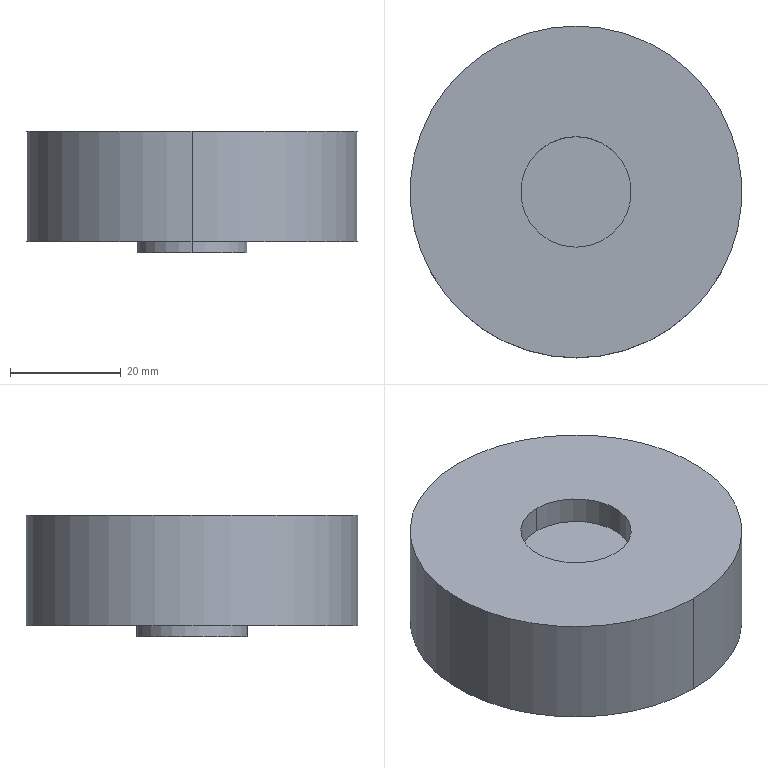Part | STEP file | B-PRF60 internal ring gear_first-stage internal ring gear | 1 solid | 10 faces | box 60 x 60 x 22 mm | volume 55606 mm3 | cylinder 6 | plane 4 | commonest cylinder face diameters 20 x4 60 x2
STEP:
#1=CARTESIAN_POINT('',(0.,0.,0.));
#2=DIRECTION('',(0.,0.,1.));
#3=DIRECTION('',(1.,0.,0.));
#4=AXIS2_PLACEMENT_3D('',#1,#2,#3);
#5=CARTESIAN_POINT('',(0.,-10.,-12.));
#6=VERTEX_POINT('',#5);
#7=CARTESIAN_POINT('',(0.,10.,-12.));
#8=VERTEX_POINT('',#7);
#9=CARTESIAN_POINT('',(0.,0.,-12.));
#10=DIRECTION('',(0.,0.,1.));
#11=DIRECTION('',(0.,-1.,0.));
#12=AXIS2_PLACEMENT_3D('',#9,#10,#11);
#13=CIRCLE('',#12,10.);
#14=CARTESIAN_POINT('',(0.,0.,-12.));
#15=DIRECTION('',(0.,0.,1.));
#16=DIRECTION('',(0.,-1.,0.));
#17=AXIS2_PLACEMENT_3D('',#14,#15,#16);
#18=CYLINDRICAL_SURFACE('',#17,10.);
#19=CARTESIAN_POINT('',(0.,0.));
#20=DIRECTION('',(1.,0.));
#21=VECTOR('',#20,1.);
#22=LINE('',#19,#21);
#23=(GEOMETRIC_REPRESENTATION_CONTEXT(2)PARAMETRIC_REPRESENTATION_CONTEXT()REPRESENTATION_CONTEXT('',''));
#24=DEFINITIONAL_REPRESENTATION('',(#22),#23);
#25=PCURVE('',#18,#24);
#26=CARTESIAN_POINT('',(0.,0.,-12.));
#27=DIRECTION('',(0.,0.,-1.));
#28=DIRECTION('',(-1.,0.,0.));
#29=AXIS2_PLACEMENT_3D('',#26,#27,#28);
#30=PLANE('',#29);
#31=CARTESIAN_POINT('',(0.,-10.));
#32=CARTESIAN_POINT('',(-17.321,-10.));
#33=CARTESIAN_POINT('',(-8.66,5.));
#34=CARTESIAN_POINT('',(0.,20.));
#35=CARTESIAN_POINT('',(8.66,5.));
#36=CARTESIAN_POINT('',(17.321,-10.));
#37=CARTESIAN_POINT('',(0.,-10.));
#38=(BOUNDED_CURVE()B_SPLINE_CURVE(2,(#31,#32,#33,#34,#35,#36,#37),.UNSPECIFIED.,.T.,.F.)B_SPLINE_CURVE_WITH_KNOTS((1,2,2,2,2,1),(-2.094,0.,2.094,4.189,6.283,8.378),.UNSPECIFIED.)CURVE()GEOMETRIC_REPRESENTATION_ITEM()RATIONAL_B_SPLINE_CURVE((1.,0.5,1.,0.5,1.,0.5,1.))REPRESENTATION_ITEM(''));
#39=(GEOMETRIC_REPRESENTATION_CONTEXT(2)PARAMETRIC_REPRESENTATION_CONTEXT()REPRESENTATION_CONTEXT('',''));
#40=DEFINITIONAL_REPRESENTATION('',(#38),#39);
#41=PCURVE('',#30,#40);
#42=SURFACE_CURVE('',#13,(#25,#41),.PCURVE_S1.);
#43=EDGE_CURVE('',#6,#8,#42,.T.);
#44=ORIENTED_EDGE('',*,*,#43,.T.);
#45=CARTESIAN_POINT('',(0.,10.,-10.));
#46=VERTEX_POINT('',#45);
#47=CARTESIAN_POINT('',(0.,10.,-12.));
#48=DIRECTION('',(0.,0.,1.));
#49=VECTOR('',#48,1.);
#50=LINE('',#47,#49);
#51=CARTESIAN_POINT('',(3.142,0.));
#52=DIRECTION('',(0.,1.));
#53=VECTOR('',#52,1.);
#54=LINE('',#51,#53);
#55=(GEOMETRIC_REPRESENTATION_CONTEXT(2)PARAMETRIC_REPRESENTATION_CONTEXT()REPRESENTATION_CONTEXT('',''));
#56=DEFINITIONAL_REPRESENTATION('',(#54),#55);
#57=PCURVE('',#18,#56);
#58=CARTESIAN_POINT('',(0.,0.,-12.));
#59=DIRECTION('',(0.,0.,1.));
#60=DIRECTION('',(0.,-1.,0.));
#61=AXIS2_PLACEMENT_3D('',#58,#59,#60);
#62=CYLINDRICAL_SURFACE('',#61,10.);
#63=CARTESIAN_POINT('',(3.142,0.));
#64=DIRECTION('',(0.,1.));
#65=VECTOR('',#64,1.);
#66=LINE('',#63,#65);
#67=(GEOMETRIC_REPRESENTATION_CONTEXT(2)PARAMETRIC_REPRESENTATION_CONTEXT()REPRESENTATION_CONTEXT('',''));
#68=DEFINITIONAL_REPRESENTATION('',(#66),#67);
#69=PCURVE('',#62,#68);
#70=SURFACE_CURVE('',#50,(#57,#69),.PCURVE_S1.);
#71=EDGE_CURVE('',#8,#46,#70,.T.);
#72=ORIENTED_EDGE('',*,*,#71,.T.);
#73=CARTESIAN_POINT('',(0.,-10.,-10.));
#74=VERTEX_POINT('',#73);
#75=CARTESIAN_POINT('',(0.,0.,-10.));
#76=DIRECTION('',(0.,0.,-1.));
#77=DIRECTION('',(0.,-1.,0.));
#78=AXIS2_PLACEMENT_3D('',#75,#76,#77);
#79=CIRCLE('',#78,10.);
#80=CARTESIAN_POINT('',(6.283,2.));
#81=DIRECTION('',(-1.,0.));
#82=VECTOR('',#81,1.);
#83=LINE('',#80,#82);
#84=(GEOMETRIC_REPRESENTATION_CONTEXT(2)PARAMETRIC_REPRESENTATION_CONTEXT()REPRESENTATION_CONTEXT('',''));
#85=DEFINITIONAL_REPRESENTATION('',(#83),#84);
#86=PCURVE('',#18,#85);
#87=CARTESIAN_POINT('',(0.,0.,-10.));
#88=DIRECTION('',(0.,0.,1.));
#89=DIRECTION('',(1.,0.,0.));
#90=AXIS2_PLACEMENT_3D('',#87,#88,#89);
#91=PLANE('',#90);
#92=CARTESIAN_POINT('',(0.,-10.));
#93=CARTESIAN_POINT('',(-17.321,-10.));
#94=CARTESIAN_POINT('',(-8.66,5.));
#95=CARTESIAN_POINT('',(0.,20.));
#96=CARTESIAN_POINT('',(8.66,5.));
#97=CARTESIAN_POINT('',(17.321,-10.));
#98=CARTESIAN_POINT('',(0.,-10.));
#99=(BOUNDED_CURVE()B_SPLINE_CURVE(2,(#92,#93,#94,#95,#96,#97,#98),.UNSPECIFIED.,.T.,.F.)B_SPLINE_CURVE_WITH_KNOTS((1,2,2,2,2,1),(-2.094,0.,2.094,4.189,6.283,8.378),.UNSPECIFIED.)CURVE()GEOMETRIC_REPRESENTATION_ITEM()RATIONAL_B_SPLINE_CURVE((1.,0.5,1.,0.5,1.,0.5,1.))REPRESENTATION_ITEM(''));
#100=(GEOMETRIC_REPRESENTATION_CONTEXT(2)PARAMETRIC_REPRESENTATION_CONTEXT()REPRESENTATION_CONTEXT('',''));
#101=DEFINITIONAL_REPRESENTATION('',(#99),#100);
#102=PCURVE('',#91,#101);
#103=SURFACE_CURVE('',#79,(#86,#102),.PCURVE_S1.);
#104=EDGE_CURVE('',#46,#74,#103,.T.);
#105=ORIENTED_EDGE('',*,*,#104,.T.);
#106=CARTESIAN_POINT('',(0.,-10.,-12.));
#107=DIRECTION('',(0.,0.,1.));
#108=VECTOR('',#107,1.);
#109=LINE('',#106,#108);
#110=CARTESIAN_POINT('',(0.,0.));
#111=DIRECTION('',(0.,1.));
#112=VECTOR('',#111,1.);
#113=LINE('',#110,#112);
#114=(GEOMETRIC_REPRESENTATION_CONTEXT(2)PARAMETRIC_REPRESENTATION_CONTEXT()REPRESENTATION_CONTEXT('',''));
#115=DEFINITIONAL_REPRESENTATION('',(#113),#114);
#116=PCURVE('',#18,#115);
#117=CARTESIAN_POINT('',(6.283,0.));
#118=DIRECTION('',(0.,1.));
#119=VECTOR('',#118,1.);
#120=LINE('',#117,#119);
#121=(GEOMETRIC_REPRESENTATION_CONTEXT(2)PARAMETRIC_REPRESENTATION_CONTEXT()REPRESENTATION_CONTEXT('',''));
#122=DEFINITIONAL_REPRESENTATION('',(#120),#121);
#123=PCURVE('',#62,#122);
#124=SURFACE_CURVE('',#109,(#116,#123),.PCURVE_S1.);
#125=EDGE_CURVE('',#6,#74,#124,.T.);
#126=ORIENTED_EDGE('',*,*,#125,.F.);
#127=EDGE_LOOP('',(#44,#72,#105,#126));
#128=FACE_BOUND('',#127,.T.);
#129=ADVANCED_FACE('',(#128),#18,.T.);
#130=CARTESIAN_POINT('',(0.,30.,10.));
#131=VERTEX_POINT('',#130);
#132=CARTESIAN_POINT('',(0.,-30.,10.));
#133=VERTEX_POINT('',#132);
#134=CARTESIAN_POINT('',(0.,0.,10.));
#135=DIRECTION('',(0.,0.,-1.));
#136=DIRECTION('',(0.,1.,0.));
#137=AXIS2_PLACEMENT_3D('',#134,#135,#136);
#138=CIRCLE('',#137,30.);
#139=CARTESIAN_POINT('',(0.,0.,10.));
#140=DIRECTION('',(0.,0.,-1.));
#141=DIRECTION('',(0.,1.,0.));
#142=AXIS2_PLACEMENT_3D('',#139,#140,#141);
#143=CYLINDRICAL_SURFACE('',#142,30.);
#144=CARTESIAN_POINT('',(0.,0.));
#145=DIRECTION('',(1.,0.));
#146=VECTOR('',#145,1.);
#147=LINE('',#144,#146);
#148=(GEOMETRIC_REPRESENTATION_CONTEXT(2)PARAMETRIC_REPRESENTATION_CONTEXT()REPRESENTATION_CONTEXT('',''));
#149=DEFINITIONAL_REPRESENTATION('',(#147),#148);
#150=PCURVE('',#143,#149);
#151=CARTESIAN_POINT('',(0.,0.,10.));
#152=DIRECTION('',(0.,0.,1.));
#153=DIRECTION('',(1.,0.,0.));
#154=AXIS2_PLACEMENT_3D('',#151,#152,#153);
#155=PLANE('',#154);
#156=CARTESIAN_POINT('',(0.,30.));
#157=CARTESIAN_POINT('',(51.962,30.));
#158=CARTESIAN_POINT('',(25.981,-15.));
#159=CARTESIAN_POINT('',(0.,-60.));
#160=CARTESIAN_POINT('',(-25.981,-15.));
#161=CARTESIAN_POINT('',(-51.962,30.));
#162=CARTESIAN_POINT('',(0.,30.));
#163=(BOUNDED_CURVE()B_SPLINE_CURVE(2,(#156,#157,#158,#159,#160,#161,#162),.UNSPECIFIED.,.T.,.F.)B_SPLINE_CURVE_WITH_KNOTS((1,2,2,2,2,1),(-2.094,0.,2.094,4.189,6.283,8.378),.UNSPECIFIED.)CURVE()GEOMETRIC_REPRESENTATION_ITEM()RATIONAL_B_SPLINE_CURVE((1.,0.5,1.,0.5,1.,0.5,1.))REPRESENTATION_ITEM(''));
#164=(GEOMETRIC_REPRESENTATION_CONTEXT(2)PARAMETRIC_REPRESENTATION_CONTEXT()REPRESENTATION_CONTEXT('',''));
#165=DEFINITIONAL_REPRESENTATION('',(#163),#164);
#166=PCURVE('',#155,#165);
#167=SURFACE_CURVE('',#138,(#150,#166),.PCURVE_S1.);
#168=EDGE_CURVE('',#131,#133,#167,.T.);
#169=ORIENTED_EDGE('',*,*,#168,.T.);
#170=CARTESIAN_POINT('',(0.,-30.,-10.));
#171=VERTEX_POINT('',#170);
#172=CARTESIAN_POINT('',(0.,-30.,10.));
#173=DIRECTION('',(0.,0.,-1.));
#174=VECTOR('',#173,1.);
#175=LINE('',#172,#174);
#176=CARTESIAN_POINT('',(3.142,0.));
#177=DIRECTION('',(0.,1.));
#178=VECTOR('',#177,1.);
#179=LINE('',#176,#178);
#180=(GEOMETRIC_REPRESENTATION_CONTEXT(2)PARAMETRIC_REPRESENTATION_CONTEXT()REPRESENTATION_CONTEXT('',''));
#181=DEFINITIONAL_REPRESENTATION('',(#179),#180);
#182=PCURVE('',#143,#181);
#183=CARTESIAN_POINT('',(0.,0.,10.));
#184=DIRECTION('',(0.,0.,-1.));
#185=DIRECTION('',(0.,1.,0.));
#186=AXIS2_PLACEMENT_3D('',#183,#184,#185);
#187=CYLINDRICAL_SURFACE('',#186,30.);
#188=CARTESIAN_POINT('',(3.142,0.));
#189=DIRECTION('',(0.,1.));
#190=VECTOR('',#189,1.);
#191=LINE('',#188,#190);
#192=(GEOMETRIC_REPRESENTATION_CONTEXT(2)PARAMETRIC_REPRESENTATION_CONTEXT()REPRESENTATION_CONTEXT('',''));
#193=DEFINITIONAL_REPRESENTATION('',(#191),#192);
#194=PCURVE('',#187,#193);
#195=SURFACE_CURVE('',#175,(#182,#194),.PCURVE_S1.);
#196=EDGE_CURVE('',#133,#171,#195,.T.);
#197=ORIENTED_EDGE('',*,*,#196,.T.);
#198=CARTESIAN_POINT('',(0.,30.,-10.));
#199=VERTEX_POINT('',#198);
#200=CARTESIAN_POINT('',(0.,0.,-10.));
#201=DIRECTION('',(0.,0.,1.));
#202=DIRECTION('',(0.,1.,0.));
#203=AXIS2_PLACEMENT_3D('',#200,#201,#202);
#204=CIRCLE('',#203,30.);
#205=CARTESIAN_POINT('',(6.283,20.));
#206=DIRECTION('',(-1.,0.));
#207=VECTOR('',#206,1.);
#208=LINE('',#205,#207);
#209=(GEOMETRIC_REPRESENTATION_CONTEXT(2)PARAMETRIC_REPRESENTATION_CONTEXT()REPRESENTATION_CONTEXT('',''));
#210=DEFINITIONAL_REPRESENTATION('',(#208),#209);
#211=PCURVE('',#143,#210);
#212=CARTESIAN_POINT('',(0.,0.));
#213=DIRECTION('',(0.,1.));
#214=AXIS2_PLACEMENT_2D('',#212,#213);
#215=CIRCLE('',#214,30.);
#216=(GEOMETRIC_REPRESENTATION_CONTEXT(2)PARAMETRIC_REPRESENTATION_CONTEXT()REPRESENTATION_CONTEXT('',''));
#217=DEFINITIONAL_REPRESENTATION('',(#215),#216);
#218=PCURVE('',#91,#217);
#219=SURFACE_CURVE('',#204,(#211,#218),.PCURVE_S1.);
#220=EDGE_CURVE('',#171,#199,#219,.T.);
#221=ORIENTED_EDGE('',*,*,#220,.T.);
#222=CARTESIAN_POINT('',(0.,30.,10.));
#223=DIRECTION('',(0.,0.,-1.));
#224=VECTOR('',#223,1.);
#225=LINE('',#222,#224);
#226=CARTESIAN_POINT('',(0.,0.));
#227=DIRECTION('',(0.,1.));
#228=VECTOR('',#227,1.);
#229=LINE('',#226,#228);
#230=(GEOMETRIC_REPRESENTATION_CONTEXT(2)PARAMETRIC_REPRESENTATION_CONTEXT()REPRESENTATION_CONTEXT('',''));
#231=DEFINITIONAL_REPRESENTATION('',(#229),#230);
#232=PCURVE('',#143,#231);
#233=CARTESIAN_POINT('',(6.283,0.));
#234=DIRECTION('',(0.,1.));
#235=VECTOR('',#234,1.);
#236=LINE('',#233,#235);
#237=(GEOMETRIC_REPRESENTATION_CONTEXT(2)PARAMETRIC_REPRESENTATION_CONTEXT()REPRESENTATION_CONTEXT('',''));
#238=DEFINITIONAL_REPRESENTATION('',(#236),#237);
#239=PCURVE('',#187,#238);
#240=SURFACE_CURVE('',#225,(#232,#239),.PCURVE_S1.);
#241=EDGE_CURVE('',#131,#199,#240,.T.);
#242=ORIENTED_EDGE('',*,*,#241,.F.);
#243=EDGE_LOOP('',(#169,#197,#221,#242));
#244=FACE_BOUND('',#243,.T.);
#245=ADVANCED_FACE('',(#244),#143,.T.);
#246=CARTESIAN_POINT('',(0.,-10.,5.));
#247=VERTEX_POINT('',#246);
#248=CARTESIAN_POINT('',(0.,-10.,10.));
#249=VERTEX_POINT('',#248);
#250=CARTESIAN_POINT('',(0.,-10.,5.));
#251=DIRECTION('',(0.,0.,1.));
#252=VECTOR('',#251,1.);
#253=LINE('',#250,#252);
#254=CARTESIAN_POINT('',(0.,0.,5.));
#255=DIRECTION('',(0.,0.,1.));
#256=DIRECTION('',(0.,-1.,0.));
#257=AXIS2_PLACEMENT_3D('',#254,#255,#256);
#258=CYLINDRICAL_SURFACE('',#257,10.);
#259=CARTESIAN_POINT('',(6.283,0.));
#260=DIRECTION('',(0.,1.));
#261=VECTOR('',#260,1.);
#262=LINE('',#259,#261);
#263=(GEOMETRIC_REPRESENTATION_CONTEXT(2)PARAMETRIC_REPRESENTATION_CONTEXT()REPRESENTATION_CONTEXT('',''));
#264=DEFINITIONAL_REPRESENTATION('',(#262),#263);
#265=PCURVE('',#258,#264);
#266=CARTESIAN_POINT('',(0.,0.,5.));
#267=DIRECTION('',(0.,0.,1.));
#268=DIRECTION('',(0.,-1.,0.));
#269=AXIS2_PLACEMENT_3D('',#266,#267,#268);
#270=CYLINDRICAL_SURFACE('',#269,10.);
#271=CARTESIAN_POINT('',(0.,0.));
#272=DIRECTION('',(0.,1.));
#273=VECTOR('',#272,1.);
#274=LINE('',#271,#273);
#275=(GEOMETRIC_REPRESENTATION_CONTEXT(2)PARAMETRIC_REPRESENTATION_CONTEXT()REPRESENTATION_CONTEXT('',''));
#276=DEFINITIONAL_REPRESENTATION('',(#274),#275);
#277=PCURVE('',#270,#276);
#278=SURFACE_CURVE('',#253,(#265,#277),.PCURVE_S1.);
#279=EDGE_CURVE('',#247,#249,#278,.T.);
#280=ORIENTED_EDGE('',*,*,#279,.T.);
#281=CARTESIAN_POINT('',(0.,10.,10.));
#282=VERTEX_POINT('',#281);
#283=CARTESIAN_POINT('',(0.,0.,10.));
#284=DIRECTION('',(0.,0.,-1.));
#285=DIRECTION('',(0.,-1.,0.));
#286=AXIS2_PLACEMENT_3D('',#283,#284,#285);
#287=CIRCLE('',#286,10.);
#288=CARTESIAN_POINT('',(6.283,5.));
#289=DIRECTION('',(-1.,0.));
#290=VECTOR('',#289,1.);
#291=LINE('',#288,#290);
#292=(GEOMETRIC_REPRESENTATION_CONTEXT(2)PARAMETRIC_REPRESENTATION_CONTEXT()REPRESENTATION_CONTEXT('',''));
#293=DEFINITIONAL_REPRESENTATION('',(#291),#292);
#294=PCURVE('',#258,#293);
#295=CARTESIAN_POINT('',(0.,-10.));
#296=CARTESIAN_POINT('',(-17.321,-10.));
#297=CARTESIAN_POINT('',(-8.66,5.));
#298=CARTESIAN_POINT('',(0.,20.));
#299=CARTESIAN_POINT('',(8.66,5.));
#300=CARTESIAN_POINT('',(17.321,-10.));
#301=CARTESIAN_POINT('',(0.,-10.));
#302=(BOUNDED_CURVE()B_SPLINE_CURVE(2,(#295,#296,#297,#298,#299,#300,#301),.UNSPECIFIED.,.T.,.F.)B_SPLINE_CURVE_WITH_KNOTS((1,2,2,2,2,1),(-2.094,0.,2.094,4.189,6.283,8.378),.UNSPECIFIED.)CURVE()GEOMETRIC_REPRESENTATION_ITEM()RATIONAL_B_SPLINE_CURVE((1.,0.5,1.,0.5,1.,0.5,1.))REPRESENTATION_ITEM(''));
#303=(GEOMETRIC_REPRESENTATION_CONTEXT(2)PARAMETRIC_REPRESENTATION_CONTEXT()REPRESENTATION_CONTEXT('',''));
#304=DEFINITIONAL_REPRESENTATION('',(#302),#303);
#305=PCURVE('',#155,#304);
#306=SURFACE_CURVE('',#287,(#294,#305),.PCURVE_S1.);
#307=EDGE_CURVE('',#249,#282,#306,.T.);
#308=ORIENTED_EDGE('',*,*,#307,.T.);
#309=CARTESIAN_POINT('',(0.,10.,5.));
#310=VERTEX_POINT('',#309);
#311=CARTESIAN_POINT('',(0.,10.,5.));
#312=DIRECTION('',(0.,0.,1.));
#313=VECTOR('',#312,1.);
#314=LINE('',#311,#313);
#315=CARTESIAN_POINT('',(3.142,0.));
#316=DIRECTION('',(0.,1.));
#317=VECTOR('',#316,1.);
#318=LINE('',#315,#317);
#319=(GEOMETRIC_REPRESENTATION_CONTEXT(2)PARAMETRIC_REPRESENTATION_CONTEXT()REPRESENTATION_CONTEXT('',''));
#320=DEFINITIONAL_REPRESENTATION('',(#318),#319);
#321=PCURVE('',#258,#320);
#322=CARTESIAN_POINT('',(3.142,0.));
#323=DIRECTION('',(0.,1.));
#324=VECTOR('',#323,1.);
#325=LINE('',#322,#324);
#326=(GEOMETRIC_REPRESENTATION_CONTEXT(2)PARAMETRIC_REPRESENTATION_CONTEXT()REPRESENTATION_CONTEXT('',''));
#327=DEFINITIONAL_REPRESENTATION('',(#325),#326);
#328=PCURVE('',#270,#327);
#329=SURFACE_CURVE('',#314,(#321,#328),.PCURVE_S1.);
#330=EDGE_CURVE('',#310,#282,#329,.T.);
#331=ORIENTED_EDGE('',*,*,#330,.F.);
#332=CARTESIAN_POINT('',(0.,0.,5.));
#333=DIRECTION('',(0.,0.,1.));
#334=DIRECTION('',(0.,-1.,0.));
#335=AXIS2_PLACEMENT_3D('',#332,#333,#334);
#336=CIRCLE('',#335,10.);
#337=CARTESIAN_POINT('',(0.,0.));
#338=DIRECTION('',(1.,0.));
#339=VECTOR('',#338,1.);
#340=LINE('',#337,#339);
#341=(GEOMETRIC_REPRESENTATION_CONTEXT(2)PARAMETRIC_REPRESENTATION_CONTEXT()REPRESENTATION_CONTEXT('',''));
#342=DEFINITIONAL_REPRESENTATION('',(#340),#341);
#343=PCURVE('',#258,#342);
#344=CARTESIAN_POINT('',(0.,0.,5.));
#345=DIRECTION('',(0.,0.,1.));
#346=DIRECTION('',(1.,0.,0.));
#347=AXIS2_PLACEMENT_3D('',#344,#345,#346);
#348=PLANE('',#347);
#349=CARTESIAN_POINT('',(0.,0.));
#350=DIRECTION('',(0.,-1.));
#351=AXIS2_PLACEMENT_2D('',#349,#350);
#352=CIRCLE('',#351,10.);
#353=(GEOMETRIC_REPRESENTATION_CONTEXT(2)PARAMETRIC_REPRESENTATION_CONTEXT()REPRESENTATION_CONTEXT('',''));
#354=DEFINITIONAL_REPRESENTATION('',(#352),#353);
#355=PCURVE('',#348,#354);
#356=SURFACE_CURVE('',#336,(#343,#355),.PCURVE_S1.);
#357=EDGE_CURVE('',#310,#247,#356,.T.);
#358=ORIENTED_EDGE('',*,*,#357,.T.);
#359=EDGE_LOOP('',(#280,#308,#331,#358));
#360=FACE_BOUND('',#359,.F.);
#361=ADVANCED_FACE('',(#360),#258,.F.);
#362=CARTESIAN_POINT('',(0.,0.,-10.));
#363=DIRECTION('',(0.,0.,-1.));
#364=DIRECTION('',(0.,-1.,0.));
#365=AXIS2_PLACEMENT_3D('',#362,#363,#364);
#366=CIRCLE('',#365,10.);
#367=CARTESIAN_POINT('',(0.,-10.));
#368=CARTESIAN_POINT('',(-17.321,-10.));
#369=CARTESIAN_POINT('',(-8.66,5.));
#370=CARTESIAN_POINT('',(0.,20.));
#371=CARTESIAN_POINT('',(8.66,5.));
#372=CARTESIAN_POINT('',(17.321,-10.));
#373=CARTESIAN_POINT('',(0.,-10.));
#374=(BOUNDED_CURVE()B_SPLINE_CURVE(2,(#367,#368,#369,#370,#371,#372,#373),.UNSPECIFIED.,.T.,.F.)B_SPLINE_CURVE_WITH_KNOTS((1,2,2,2,2,1),(-2.094,0.,2.094,4.189,6.283,8.378),.UNSPECIFIED.)CURVE()GEOMETRIC_REPRESENTATION_ITEM()RATIONAL_B_SPLINE_CURVE((1.,0.5,1.,0.5,1.,0.5,1.))REPRESENTATION_ITEM(''));
#375=(GEOMETRIC_REPRESENTATION_CONTEXT(2)PARAMETRIC_REPRESENTATION_CONTEXT()REPRESENTATION_CONTEXT('',''));
#376=DEFINITIONAL_REPRESENTATION('',(#374),#375);
#377=PCURVE('',#91,#376);
#378=CARTESIAN_POINT('',(6.283,2.));
#379=DIRECTION('',(-1.,0.));
#380=VECTOR('',#379,1.);
#381=LINE('',#378,#380);
#382=(GEOMETRIC_REPRESENTATION_CONTEXT(2)PARAMETRIC_REPRESENTATION_CONTEXT()REPRESENTATION_CONTEXT('',''));
#383=DEFINITIONAL_REPRESENTATION('',(#381),#382);
#384=PCURVE('',#62,#383);
#385=SURFACE_CURVE('',#366,(#377,#384),.PCURVE_S1.);
#386=EDGE_CURVE('',#74,#46,#385,.T.);
#387=ORIENTED_EDGE('',*,*,#386,.F.);
#388=ORIENTED_EDGE('',*,*,#104,.F.);
#389=EDGE_LOOP('',(#387,#388));
#390=FACE_BOUND('',#389,.T.);
#391=CARTESIAN_POINT('',(0.,0.,-10.));
#392=DIRECTION('',(0.,0.,1.));
#393=DIRECTION('',(0.,1.,0.));
#394=AXIS2_PLACEMENT_3D('',#391,#392,#393);
#395=CIRCLE('',#394,30.);
#396=CARTESIAN_POINT('',(0.,0.));
#397=DIRECTION('',(0.,1.));
#398=AXIS2_PLACEMENT_2D('',#396,#397);
#399=CIRCLE('',#398,30.);
#400=(GEOMETRIC_REPRESENTATION_CONTEXT(2)PARAMETRIC_REPRESENTATION_CONTEXT()REPRESENTATION_CONTEXT('',''));
#401=DEFINITIONAL_REPRESENTATION('',(#399),#400);
#402=PCURVE('',#91,#401);
#403=CARTESIAN_POINT('',(6.283,20.));
#404=DIRECTION('',(-1.,0.));
#405=VECTOR('',#404,1.);
#406=LINE('',#403,#405);
#407=(GEOMETRIC_REPRESENTATION_CONTEXT(2)PARAMETRIC_REPRESENTATION_CONTEXT()REPRESENTATION_CONTEXT('',''));
#408=DEFINITIONAL_REPRESENTATION('',(#406),#407);
#409=PCURVE('',#187,#408);
#410=SURFACE_CURVE('',#395,(#402,#409),.PCURVE_S1.);
#411=EDGE_CURVE('',#199,#171,#410,.T.);
#412=ORIENTED_EDGE('',*,*,#411,.F.);
#413=ORIENTED_EDGE('',*,*,#220,.F.);
#414=EDGE_LOOP('',(#412,#413));
#415=FACE_BOUND('',#414,.T.);
#416=ADVANCED_FACE('',(#390,#415),#91,.F.);
#417=ORIENTED_EDGE('',*,*,#71,.F.);
#418=CARTESIAN_POINT('',(0.,0.,-12.));
#419=DIRECTION('',(0.,0.,1.));
#420=DIRECTION('',(0.,-1.,0.));
#421=AXIS2_PLACEMENT_3D('',#418,#419,#420);
#422=CIRCLE('',#421,10.);
#423=CARTESIAN_POINT('',(0.,0.));
#424=DIRECTION('',(1.,0.));
#425=VECTOR('',#424,1.);
#426=LINE('',#423,#425);
#427=(GEOMETRIC_REPRESENTATION_CONTEXT(2)PARAMETRIC_REPRESENTATION_CONTEXT()REPRESENTATION_CONTEXT('',''));
#428=DEFINITIONAL_REPRESENTATION('',(#426),#427);
#429=PCURVE('',#62,#428);
#430=CARTESIAN_POINT('',(0.,-10.));
#431=CARTESIAN_POINT('',(-17.321,-10.));
#432=CARTESIAN_POINT('',(-8.66,5.));
#433=CARTESIAN_POINT('',(0.,20.));
#434=CARTESIAN_POINT('',(8.66,5.));
#435=CARTESIAN_POINT('',(17.321,-10.));
#436=CARTESIAN_POINT('',(0.,-10.));
#437=(BOUNDED_CURVE()B_SPLINE_CURVE(2,(#430,#431,#432,#433,#434,#435,#436),.UNSPECIFIED.,.T.,.F.)B_SPLINE_CURVE_WITH_KNOTS((1,2,2,2,2,1),(-2.094,0.,2.094,4.189,6.283,8.378),.UNSPECIFIED.)CURVE()GEOMETRIC_REPRESENTATION_ITEM()RATIONAL_B_SPLINE_CURVE((1.,0.5,1.,0.5,1.,0.5,1.))REPRESENTATION_ITEM(''));
#438=(GEOMETRIC_REPRESENTATION_CONTEXT(2)PARAMETRIC_REPRESENTATION_CONTEXT()REPRESENTATION_CONTEXT('',''));
#439=DEFINITIONAL_REPRESENTATION('',(#437),#438);
#440=PCURVE('',#30,#439);
#441=SURFACE_CURVE('',#422,(#429,#440),.PCURVE_S1.);
#442=EDGE_CURVE('',#8,#6,#441,.T.);
#443=ORIENTED_EDGE('',*,*,#442,.T.);
#444=ORIENTED_EDGE('',*,*,#125,.T.);
#445=ORIENTED_EDGE('',*,*,#386,.T.);
#446=EDGE_LOOP('',(#417,#443,#444,#445));
#447=FACE_BOUND('',#446,.T.);
#448=ADVANCED_FACE('',(#447),#62,.T.);
#449=ORIENTED_EDGE('',*,*,#196,.F.);
#450=CARTESIAN_POINT('',(0.,0.,10.));
#451=DIRECTION('',(0.,0.,-1.));
#452=DIRECTION('',(0.,1.,0.));
#453=AXIS2_PLACEMENT_3D('',#450,#451,#452);
#454=CIRCLE('',#453,30.);
#455=CARTESIAN_POINT('',(0.,0.));
#456=DIRECTION('',(1.,0.));
#457=VECTOR('',#456,1.);
#458=LINE('',#455,#457);
#459=(GEOMETRIC_REPRESENTATION_CONTEXT(2)PARAMETRIC_REPRESENTATION_CONTEXT()REPRESENTATION_CONTEXT('',''));
#460=DEFINITIONAL_REPRESENTATION('',(#458),#459);
#461=PCURVE('',#187,#460);
#462=CARTESIAN_POINT('',(0.,30.));
#463=CARTESIAN_POINT('',(51.962,30.));
#464=CARTESIAN_POINT('',(25.981,-15.));
#465=CARTESIAN_POINT('',(0.,-60.));
#466=CARTESIAN_POINT('',(-25.981,-15.));
#467=CARTESIAN_POINT('',(-51.962,30.));
#468=CARTESIAN_POINT('',(0.,30.));
#469=(BOUNDED_CURVE()B_SPLINE_CURVE(2,(#462,#463,#464,#465,#466,#467,#468),.UNSPECIFIED.,.T.,.F.)B_SPLINE_CURVE_WITH_KNOTS((1,2,2,2,2,1),(-2.094,0.,2.094,4.189,6.283,8.378),.UNSPECIFIED.)CURVE()GEOMETRIC_REPRESENTATION_ITEM()RATIONAL_B_SPLINE_CURVE((1.,0.5,1.,0.5,1.,0.5,1.))REPRESENTATION_ITEM(''));
#470=(GEOMETRIC_REPRESENTATION_CONTEXT(2)PARAMETRIC_REPRESENTATION_CONTEXT()REPRESENTATION_CONTEXT('',''));
#471=DEFINITIONAL_REPRESENTATION('',(#469),#470);
#472=PCURVE('',#155,#471);
#473=SURFACE_CURVE('',#454,(#461,#472),.PCURVE_S1.);
#474=EDGE_CURVE('',#133,#131,#473,.T.);
#475=ORIENTED_EDGE('',*,*,#474,.T.);
#476=ORIENTED_EDGE('',*,*,#241,.T.);
#477=ORIENTED_EDGE('',*,*,#411,.T.);
#478=EDGE_LOOP('',(#449,#475,#476,#477));
#479=FACE_BOUND('',#478,.T.);
#480=ADVANCED_FACE('',(#479),#187,.T.);
#481=ORIENTED_EDGE('',*,*,#43,.F.);
#482=ORIENTED_EDGE('',*,*,#442,.F.);
#483=EDGE_LOOP('',(#481,#482));
#484=FACE_BOUND('',#483,.T.);
#485=ADVANCED_FACE('',(#484),#30,.T.);
#486=ORIENTED_EDGE('',*,*,#168,.F.);
#487=ORIENTED_EDGE('',*,*,#474,.F.);
#488=EDGE_LOOP('',(#486,#487));
#489=FACE_BOUND('',#488,.T.);
#490=ORIENTED_EDGE('',*,*,#307,.T.);
#491=CARTESIAN_POINT('',(0.,0.,10.));
#492=DIRECTION('',(0.,0.,-1.));
#493=DIRECTION('',(0.,-1.,0.));
#494=AXIS2_PLACEMENT_3D('',#491,#492,#493);
#495=CIRCLE('',#494,10.);
#496=CARTESIAN_POINT('',(0.,-10.));
#497=CARTESIAN_POINT('',(-17.321,-10.));
#498=CARTESIAN_POINT('',(-8.66,5.));
#499=CARTESIAN_POINT('',(0.,20.));
#500=CARTESIAN_POINT('',(8.66,5.));
#501=CARTESIAN_POINT('',(17.321,-10.));
#502=CARTESIAN_POINT('',(0.,-10.));
#503=(BOUNDED_CURVE()B_SPLINE_CURVE(2,(#496,#497,#498,#499,#500,#501,#502),.UNSPECIFIED.,.T.,.F.)B_SPLINE_CURVE_WITH_KNOTS((1,2,2,2,2,1),(-2.094,0.,2.094,4.189,6.283,8.378),.UNSPECIFIED.)CURVE()GEOMETRIC_REPRESENTATION_ITEM()RATIONAL_B_SPLINE_CURVE((1.,0.5,1.,0.5,1.,0.5,1.))REPRESENTATION_ITEM(''));
#504=(GEOMETRIC_REPRESENTATION_CONTEXT(2)PARAMETRIC_REPRESENTATION_CONTEXT()REPRESENTATION_CONTEXT('',''));
#505=DEFINITIONAL_REPRESENTATION('',(#503),#504);
#506=PCURVE('',#155,#505);
#507=CARTESIAN_POINT('',(6.283,5.));
#508=DIRECTION('',(-1.,0.));
#509=VECTOR('',#508,1.);
#510=LINE('',#507,#509);
#511=(GEOMETRIC_REPRESENTATION_CONTEXT(2)PARAMETRIC_REPRESENTATION_CONTEXT()REPRESENTATION_CONTEXT('',''));
#512=DEFINITIONAL_REPRESENTATION('',(#510),#511);
#513=PCURVE('',#270,#512);
#514=SURFACE_CURVE('',#495,(#506,#513),.PCURVE_S1.);
#515=EDGE_CURVE('',#282,#249,#514,.T.);
#516=ORIENTED_EDGE('',*,*,#515,.T.);
#517=EDGE_LOOP('',(#490,#516));
#518=FACE_BOUND('',#517,.T.);
#519=ADVANCED_FACE('',(#489,#518),#155,.T.);
#520=ORIENTED_EDGE('',*,*,#515,.T.);
#521=ORIENTED_EDGE('',*,*,#279,.F.);
#522=CARTESIAN_POINT('',(0.,0.,5.));
#523=DIRECTION('',(0.,0.,1.));
#524=DIRECTION('',(0.,-1.,0.));
#525=AXIS2_PLACEMENT_3D('',#522,#523,#524);
#526=CIRCLE('',#525,10.);
#527=CARTESIAN_POINT('',(0.,0.));
#528=DIRECTION('',(1.,0.));
#529=VECTOR('',#528,1.);
#530=LINE('',#527,#529);
#531=(GEOMETRIC_REPRESENTATION_CONTEXT(2)PARAMETRIC_REPRESENTATION_CONTEXT()REPRESENTATION_CONTEXT('',''));
#532=DEFINITIONAL_REPRESENTATION('',(#530),#531);
#533=PCURVE('',#270,#532);
#534=CARTESIAN_POINT('',(0.,0.));
#535=DIRECTION('',(0.,-1.));
#536=AXIS2_PLACEMENT_2D('',#534,#535);
#537=CIRCLE('',#536,10.);
#538=(GEOMETRIC_REPRESENTATION_CONTEXT(2)PARAMETRIC_REPRESENTATION_CONTEXT()REPRESENTATION_CONTEXT('',''));
#539=DEFINITIONAL_REPRESENTATION('',(#537),#538);
#540=PCURVE('',#348,#539);
#541=SURFACE_CURVE('',#526,(#533,#540),.PCURVE_S1.);
#542=EDGE_CURVE('',#247,#310,#541,.T.);
#543=ORIENTED_EDGE('',*,*,#542,.T.);
#544=ORIENTED_EDGE('',*,*,#330,.T.);
#545=EDGE_LOOP('',(#520,#521,#543,#544));
#546=FACE_BOUND('',#545,.F.);
#547=ADVANCED_FACE('',(#546),#270,.F.);
#548=ORIENTED_EDGE('',*,*,#542,.T.);
#549=ORIENTED_EDGE('',*,*,#357,.T.);
#550=EDGE_LOOP('',(#548,#549));
#551=FACE_BOUND('',#550,.T.);
#552=ADVANCED_FACE('',(#551),#348,.T.);
#553=CLOSED_SHELL('',(#129,#245,#361,#416,#448,#480,#485,#519,#547,#552));
#554=MANIFOLD_SOLID_BREP('',#553);
#555=(LENGTH_UNIT()NAMED_UNIT(*)SI_UNIT(.MILLI.,.METRE.));
#556=UNCERTAINTY_MEASURE_WITH_UNIT(LENGTH_MEASURE(0.0000001),#555,'','');
#557=(NAMED_UNIT(*)PLANE_ANGLE_UNIT()SI_UNIT($,.RADIAN.));
#558=(NAMED_UNIT(*)SI_UNIT($,.STERADIAN.)SOLID_ANGLE_UNIT());
#559=(GEOMETRIC_REPRESENTATION_CONTEXT(3)GLOBAL_UNCERTAINTY_ASSIGNED_CONTEXT((#556))GLOBAL_UNIT_ASSIGNED_CONTEXT((#555,#557,#558))REPRESENTATION_CONTEXT('',''));
#560=ADVANCED_BREP_SHAPE_REPRESENTATION('',(#4,#554),#559);